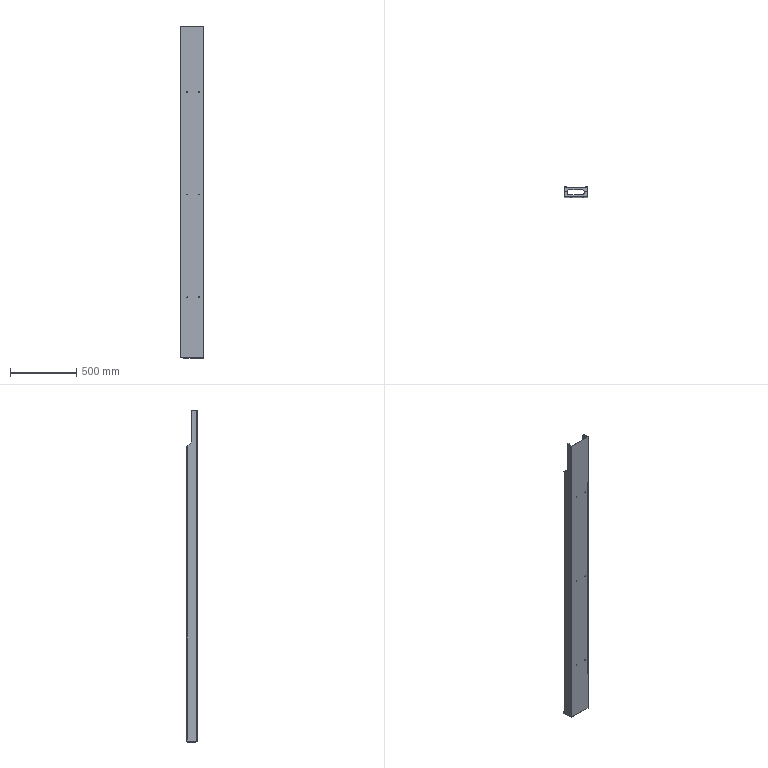Part | SolidWorks | features EdgeFlange 6, ICE 3, Cut 2, Chamfer 1, FlatPattern 1, LPattern 1, SMBaseFlange 1, SheetMetal 1 | 1 solid | 128 faces | box 180 x 80 x 2507 mm | volume 1382139 mm3 | plane 82 | cylinder 34 | cone 12 | commonest cylinder face diameters 6 x12 2 x8 5 x8 6.4 x4 40 x2